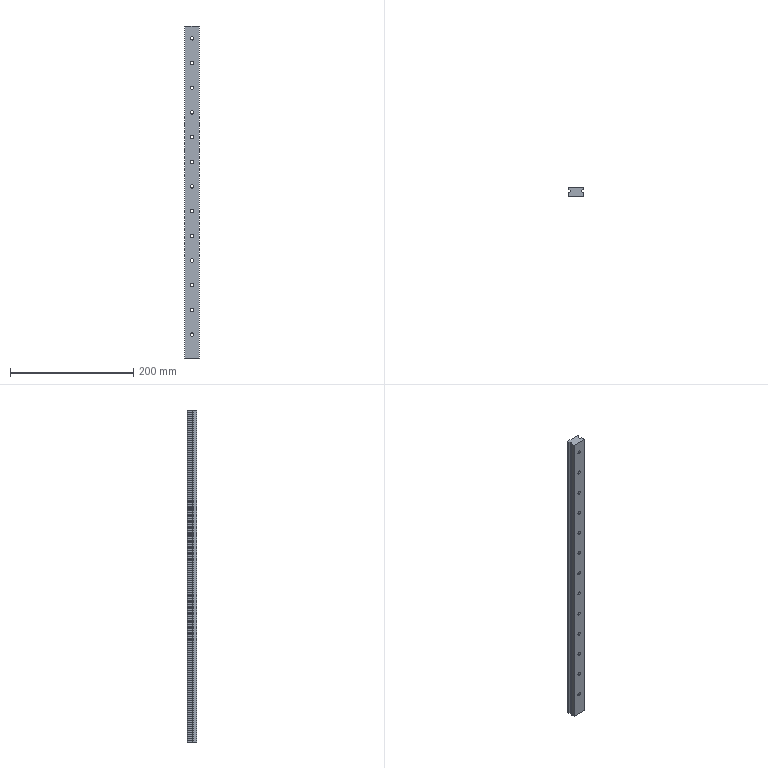Part | SolidWorks | features Extrusion 1, HoleWzd 1 | 1 solid | 115 faces | box 23.597 x 15.078 x 538 mm | volume 168139 mm3 | cylinder 62 | plane 27 | cone 26 | commonest cylinder face diameters 5.5 x26 10 x26 2 x10